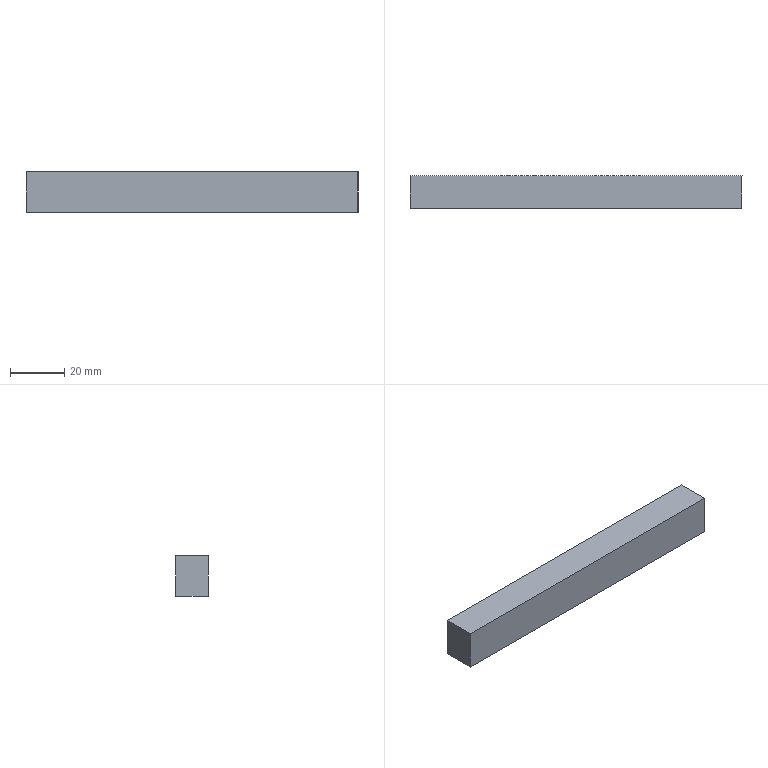Part | NX | features solid 2 | 1 solid | 6 faces | box 122 x 12 x 15 mm | volume 21960 mm3 | plane 6
STEP:
#1=CARTESIAN_POINT('',(-670.,484.,-20.));
#2=VERTEX_POINT('',#1);
#3=CARTESIAN_POINT('',(-670.,484.,-35.));
#4=VERTEX_POINT('',#3);
#5=CARTESIAN_POINT('',(-670.,484.,54.523));
#6=DIRECTION('',(0.,0.,-1.));
#7=VECTOR('',#6,1000.);
#8=LINE('',#5,#7);
#9=EDGE_CURVE('',#2,#4,#8,.T.);
#10=ORIENTED_EDGE('',*,*,#9,.F.);
#11=CARTESIAN_POINT('',(-670.,496.,-20.));
#12=VERTEX_POINT('',#11);
#13=CARTESIAN_POINT('',(-670.,463.,-20.));
#14=DIRECTION('',(0.,1.,0.));
#15=VECTOR('',#14,1000.);
#16=LINE('',#13,#15);
#17=EDGE_CURVE('',#2,#12,#16,.T.);
#18=ORIENTED_EDGE('',*,*,#17,.T.);
#19=CARTESIAN_POINT('',(-670.,496.,-35.));
#20=VERTEX_POINT('',#19);
#21=CARTESIAN_POINT('',(-670.,496.,54.523));
#22=DIRECTION('',(0.,0.,-1.));
#23=VECTOR('',#22,1000.);
#24=LINE('',#21,#23);
#25=EDGE_CURVE('',#12,#20,#24,.T.);
#26=ORIENTED_EDGE('',*,*,#25,.T.);
#27=CARTESIAN_POINT('',(-670.,463.,-35.));
#28=DIRECTION('',(0.,1.,0.));
#29=VECTOR('',#28,1000.);
#30=LINE('',#27,#29);
#31=EDGE_CURVE('',#4,#20,#30,.T.);
#32=ORIENTED_EDGE('',*,*,#31,.F.);
#33=EDGE_LOOP('',(#10,#18,#26,#32));
#34=FACE_BOUND('',#33,.T.);
#35=CARTESIAN_POINT('',(-670.,496.,-20.));
#36=DIRECTION('',(1.,0.,0.));
#37=DIRECTION('',(0.,0.,-1.));
#38=AXIS2_PLACEMENT_3D('',#35,#36,#37);
#39=PLANE('',#38);
#40=ADVANCED_FACE('',(#34),#39,.F.);
#41=CARTESIAN_POINT('',(-548.,484.,-35.));
#42=VERTEX_POINT('',#41);
#43=CARTESIAN_POINT('',(-548.,496.,-35.));
#44=VERTEX_POINT('',#43);
#45=CARTESIAN_POINT('',(-548.,463.,-35.));
#46=DIRECTION('',(0.,1.,0.));
#47=VECTOR('',#46,1000.);
#48=LINE('',#45,#47);
#49=EDGE_CURVE('',#42,#44,#48,.T.);
#50=ORIENTED_EDGE('',*,*,#49,.F.);
#51=CARTESIAN_POINT('',(-640.,484.,-35.));
#52=DIRECTION('',(-1.,0.,0.));
#53=VECTOR('',#52,1000.);
#54=LINE('',#51,#53);
#55=EDGE_CURVE('',#42,#4,#54,.T.);
#56=ORIENTED_EDGE('',*,*,#55,.T.);
#57=ORIENTED_EDGE('',*,*,#31,.T.);
#58=CARTESIAN_POINT('',(-640.,496.,-35.));
#59=DIRECTION('',(-1.,0.,0.));
#60=VECTOR('',#59,1000.);
#61=LINE('',#58,#60);
#62=EDGE_CURVE('',#44,#20,#61,.T.);
#63=ORIENTED_EDGE('',*,*,#62,.F.);
#64=EDGE_LOOP('',(#50,#56,#57,#63));
#65=FACE_BOUND('',#64,.T.);
#66=CARTESIAN_POINT('',(-623.,463.,-35.));
#67=DIRECTION('',(0.,0.,1.));
#68=DIRECTION('',(0.,1.,0.));
#69=AXIS2_PLACEMENT_3D('',#66,#67,#68);
#70=PLANE('',#69);
#71=ADVANCED_FACE('',(#65),#70,.F.);
#72=ORIENTED_EDGE('',*,*,#17,.F.);
#73=CARTESIAN_POINT('',(-548.,484.,-20.));
#74=VERTEX_POINT('',#73);
#75=CARTESIAN_POINT('',(-640.,484.,-20.));
#76=DIRECTION('',(1.,0.,0.));
#77=VECTOR('',#76,1000.);
#78=LINE('',#75,#77);
#79=EDGE_CURVE('',#2,#74,#78,.T.);
#80=ORIENTED_EDGE('',*,*,#79,.T.);
#81=CARTESIAN_POINT('',(-548.,496.,-20.));
#82=VERTEX_POINT('',#81);
#83=CARTESIAN_POINT('',(-548.,645.,-20.));
#84=DIRECTION('',(0.,1.,0.));
#85=VECTOR('',#84,1000.);
#86=LINE('',#83,#85);
#87=EDGE_CURVE('',#74,#82,#86,.T.);
#88=ORIENTED_EDGE('',*,*,#87,.T.);
#89=CARTESIAN_POINT('',(-663.,496.,-20.));
#90=DIRECTION('',(-1.,0.,0.));
#91=VECTOR('',#90,1000.);
#92=LINE('',#89,#91);
#93=EDGE_CURVE('',#82,#12,#92,.T.);
#94=ORIENTED_EDGE('',*,*,#93,.T.);
#95=EDGE_LOOP('',(#72,#80,#88,#94));
#96=FACE_BOUND('',#95,.T.);
#97=CARTESIAN_POINT('',(-623.,463.,-20.));
#98=DIRECTION('',(0.,0.,1.));
#99=DIRECTION('',(0.,1.,0.));
#100=AXIS2_PLACEMENT_3D('',#97,#98,#99);
#101=PLANE('',#100);
#102=ADVANCED_FACE('',(#96),#101,.T.);
#103=CARTESIAN_POINT('',(-548.,484.,54.523));
#104=DIRECTION('',(0.,0.,-1.));
#105=VECTOR('',#104,1000.);
#106=LINE('',#103,#105);
#107=EDGE_CURVE('',#74,#42,#106,.T.);
#108=ORIENTED_EDGE('',*,*,#107,.F.);
#109=ORIENTED_EDGE('',*,*,#79,.F.);
#110=ORIENTED_EDGE('',*,*,#9,.T.);
#111=ORIENTED_EDGE('',*,*,#55,.F.);
#112=EDGE_LOOP('',(#108,#109,#110,#111));
#113=FACE_BOUND('',#112,.T.);
#114=CARTESIAN_POINT('',(-640.,484.,54.523));
#115=DIRECTION('',(0.,1.,0.));
#116=DIRECTION('',(1.,0.,0.));
#117=AXIS2_PLACEMENT_3D('',#114,#115,#116);
#118=PLANE('',#117);
#119=ADVANCED_FACE('',(#113),#118,.F.);
#120=ORIENTED_EDGE('',*,*,#93,.F.);
#121=CARTESIAN_POINT('',(-548.,496.,54.523));
#122=DIRECTION('',(0.,0.,-1.));
#123=VECTOR('',#122,1000.);
#124=LINE('',#121,#123);
#125=EDGE_CURVE('',#82,#44,#124,.T.);
#126=ORIENTED_EDGE('',*,*,#125,.T.);
#127=ORIENTED_EDGE('',*,*,#62,.T.);
#128=ORIENTED_EDGE('',*,*,#25,.F.);
#129=EDGE_LOOP('',(#120,#126,#127,#128));
#130=FACE_BOUND('',#129,.T.);
#131=CARTESIAN_POINT('',(-640.,496.,54.523));
#132=DIRECTION('',(0.,1.,0.));
#133=DIRECTION('',(1.,0.,0.));
#134=AXIS2_PLACEMENT_3D('',#131,#132,#133);
#135=PLANE('',#134);
#136=ADVANCED_FACE('',(#130),#135,.T.);
#137=ORIENTED_EDGE('',*,*,#107,.T.);
#138=ORIENTED_EDGE('',*,*,#49,.T.);
#139=ORIENTED_EDGE('',*,*,#125,.F.);
#140=ORIENTED_EDGE('',*,*,#87,.F.);
#141=EDGE_LOOP('',(#137,#138,#139,#140));
#142=FACE_BOUND('',#141,.T.);
#143=CARTESIAN_POINT('',(-548.,496.,-20.));
#144=DIRECTION('',(1.,0.,0.));
#145=DIRECTION('',(0.,1.,0.));
#146=AXIS2_PLACEMENT_3D('',#143,#144,#145);
#147=PLANE('',#146);
#148=ADVANCED_FACE('',(#142),#147,.T.);
#149=CLOSED_SHELL('',(#40,#71,#102,#119,#136,#148));
#150=MANIFOLD_SOLID_BREP('',#149);
#151=(LENGTH_UNIT()NAMED_UNIT(*)SI_UNIT(.MILLI.,.METRE.));
#152=UNCERTAINTY_MEASURE_WITH_UNIT(LENGTH_MEASURE(0.00001),#151,'','');
#153=(NAMED_UNIT(*)PLANE_ANGLE_UNIT()SI_UNIT($,.RADIAN.));
#154=(NAMED_UNIT(*)SI_UNIT($,.STERADIAN.)SOLID_ANGLE_UNIT());
#155=(GEOMETRIC_REPRESENTATION_CONTEXT(3)GLOBAL_UNCERTAINTY_ASSIGNED_CONTEXT((#152))GLOBAL_UNIT_ASSIGNED_CONTEXT((#151,#153,#154))REPRESENTATION_CONTEXT('',''));
#156=ADVANCED_BREP_SHAPE_REPRESENTATION('',(#150),#155);